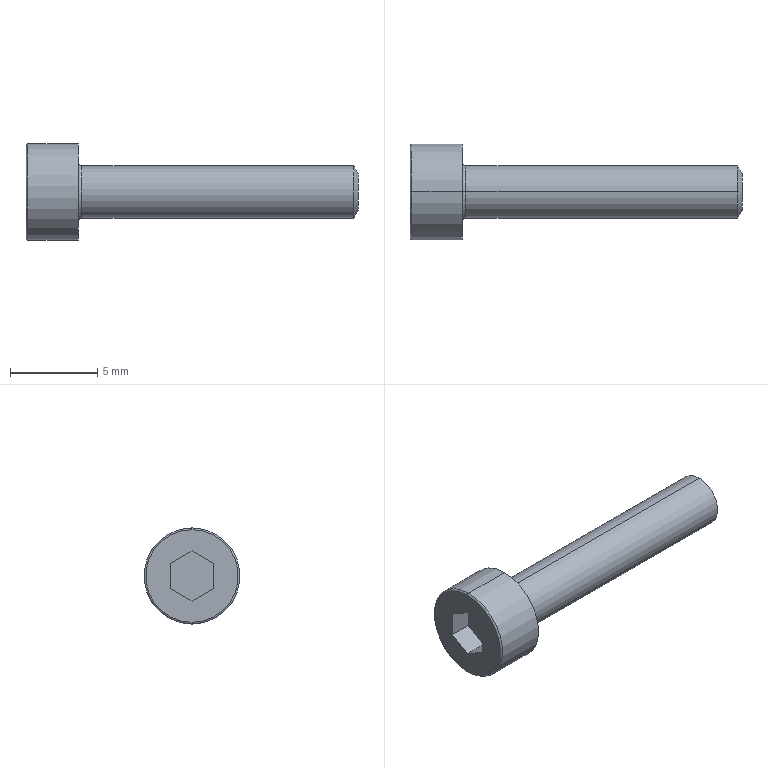Part | STEP file | 1 solid | 20 faces | box 19 x 5.5 x 5.5 mm | volume 177.003 mm3 | plane 10 | torus 4 | cylinder 4 | cone 2 | commonest cylinder face diameters 3 x2 5.5 x2
STEP:
#1=CARTESIAN_POINT('',(0.,0.,2.65));
#2=VERTEX_POINT('',#1);
#3=CARTESIAN_POINT('',(0.,0.,-2.65));
#4=VERTEX_POINT('',#3);
#5=CARTESIAN_POINT('',(0.,0.,0.));
#6=DIRECTION('',(-1.,0.,0.));
#7=DIRECTION('',(0.,0.,-1.));
#8=AXIS2_PLACEMENT_3D('',#5,#6,#7);
#9=CIRCLE('',#8,2.65);
#10=EDGE_CURVE('',#2,#4,#9,.T.);
#11=ORIENTED_EDGE('',*,*,#10,.F.);
#12=CARTESIAN_POINT('',(0.1,0.,2.75));
#13=VERTEX_POINT('',#12);
#14=CARTESIAN_POINT('',(0.1,0.,2.65));
#15=DIRECTION('',(0.,1.,0.));
#16=DIRECTION('',(0.,0.,1.));
#17=AXIS2_PLACEMENT_3D('',#14,#15,#16);
#18=CIRCLE('',#17,0.1);
#19=EDGE_CURVE('',#2,#13,#18,.T.);
#20=ORIENTED_EDGE('',*,*,#19,.T.);
#21=CARTESIAN_POINT('',(0.1,0.,-2.75));
#22=VERTEX_POINT('',#21);
#23=CARTESIAN_POINT('',(0.1,0.,0.));
#24=DIRECTION('',(1.,0.,0.));
#25=DIRECTION('',(0.,0.,-1.));
#26=AXIS2_PLACEMENT_3D('',#23,#24,#25);
#27=CIRCLE('',#26,2.75);
#28=EDGE_CURVE('',#22,#13,#27,.T.);
#29=ORIENTED_EDGE('',*,*,#28,.F.);
#30=CARTESIAN_POINT('',(0.1,0.,-2.65));
#31=DIRECTION('',(0.,-1.,0.));
#32=DIRECTION('',(0.,0.,-1.));
#33=AXIS2_PLACEMENT_3D('',#30,#31,#32);
#34=CIRCLE('',#33,0.1);
#35=EDGE_CURVE('',#4,#22,#34,.T.);
#36=ORIENTED_EDGE('',*,*,#35,.F.);
#37=EDGE_LOOP('',(#11,#20,#29,#36));
#38=FACE_OUTER_BOUND('',#37,.T.);
#39=CARTESIAN_POINT('',(0.1,0.,0.));
#40=DIRECTION('',(1.,0.,0.));
#41=DIRECTION('',(0.,0.,-1.));
#42=AXIS2_PLACEMENT_3D('',#39,#40,#41);
#43=TOROIDAL_SURFACE('',#42,2.65,0.1);
#44=ADVANCED_FACE('',(#38),#43,.T.);
#45=CARTESIAN_POINT('',(19.,0.,1.067));
#46=VERTEX_POINT('',#45);
#47=CARTESIAN_POINT('',(19.,0.,-1.067));
#48=VERTEX_POINT('',#47);
#49=CARTESIAN_POINT('',(19.,0.,0.));
#50=DIRECTION('',(-1.,0.,0.));
#51=DIRECTION('',(0.,0.,1.));
#52=AXIS2_PLACEMENT_3D('',#49,#50,#51);
#53=CIRCLE('',#52,1.067);
#54=EDGE_CURVE('',#46,#48,#53,.T.);
#55=ORIENTED_EDGE('',*,*,#54,.T.);
#56=CARTESIAN_POINT('',(18.75,0.,-1.5));
#57=VERTEX_POINT('',#56);
#58=CARTESIAN_POINT('',(18.75,0.,-1.5));
#59=DIRECTION('',(-0.5,0.,-0.866));
#60=VECTOR('',#59,1000.);
#61=LINE('',#58,#60);
#62=EDGE_CURVE('',#48,#57,#61,.T.);
#63=ORIENTED_EDGE('',*,*,#62,.T.);
#64=CARTESIAN_POINT('',(18.75,0.,1.5));
#65=VERTEX_POINT('',#64);
#66=CARTESIAN_POINT('',(18.75,0.,0.));
#67=DIRECTION('',(-1.,0.,0.));
#68=DIRECTION('',(0.,0.,1.));
#69=AXIS2_PLACEMENT_3D('',#66,#67,#68);
#70=CIRCLE('',#69,1.5);
#71=EDGE_CURVE('',#65,#57,#70,.T.);
#72=ORIENTED_EDGE('',*,*,#71,.F.);
#73=CARTESIAN_POINT('',(18.75,0.,1.5));
#74=DIRECTION('',(-0.5,0.,0.866));
#75=VECTOR('',#74,1000.);
#76=LINE('',#73,#75);
#77=EDGE_CURVE('',#46,#65,#76,.T.);
#78=ORIENTED_EDGE('',*,*,#77,.F.);
#79=EDGE_LOOP('',(#55,#63,#72,#78));
#80=FACE_OUTER_BOUND('',#79,.T.);
#81=CARTESIAN_POINT('',(18.75,0.,0.));
#82=DIRECTION('',(-1.,0.,0.));
#83=DIRECTION('',(0.,0.,1.));
#84=AXIS2_PLACEMENT_3D('',#81,#82,#83);
#85=CONICAL_SURFACE('',#84,1.5,1.047);
#86=ADVANCED_FACE('',(#80),#85,.T.);
#87=CARTESIAN_POINT('',(3.,0.,-1.7));
#88=VERTEX_POINT('',#87);
#89=CARTESIAN_POINT('',(3.,0.,1.7));
#90=VERTEX_POINT('',#89);
#91=CARTESIAN_POINT('',(3.,0.,0.));
#92=DIRECTION('',(-1.,0.,0.));
#93=DIRECTION('',(0.,0.,1.));
#94=AXIS2_PLACEMENT_3D('',#91,#92,#93);
#95=CIRCLE('',#94,1.7);
#96=EDGE_CURVE('',#88,#90,#95,.T.);
#97=ORIENTED_EDGE('',*,*,#96,.F.);
#98=CARTESIAN_POINT('',(3.2,0.,-1.5));
#99=VERTEX_POINT('',#98);
#100=CARTESIAN_POINT('',(3.2,0.,-1.7));
#101=DIRECTION('',(0.,1.,0.));
#102=DIRECTION('',(0.,0.,1.));
#103=AXIS2_PLACEMENT_3D('',#100,#101,#102);
#104=CIRCLE('',#103,0.2);
#105=EDGE_CURVE('',#88,#99,#104,.T.);
#106=ORIENTED_EDGE('',*,*,#105,.T.);
#107=CARTESIAN_POINT('',(3.2,0.,1.5));
#108=VERTEX_POINT('',#107);
#109=CARTESIAN_POINT('',(3.2,0.,0.));
#110=DIRECTION('',(-1.,0.,0.));
#111=DIRECTION('',(0.,0.,1.));
#112=AXIS2_PLACEMENT_3D('',#109,#110,#111);
#113=CIRCLE('',#112,1.5);
#114=EDGE_CURVE('',#99,#108,#113,.T.);
#115=ORIENTED_EDGE('',*,*,#114,.T.);
#116=CARTESIAN_POINT('',(3.2,0.,1.7));
#117=DIRECTION('',(0.,-1.,0.));
#118=DIRECTION('',(0.,0.,-1.));
#119=AXIS2_PLACEMENT_3D('',#116,#117,#118);
#120=CIRCLE('',#119,0.2);
#121=EDGE_CURVE('',#90,#108,#120,.T.);
#122=ORIENTED_EDGE('',*,*,#121,.F.);
#123=EDGE_LOOP('',(#97,#106,#115,#122));
#124=FACE_OUTER_BOUND('',#123,.T.);
#125=CARTESIAN_POINT('',(3.2,0.,0.));
#126=DIRECTION('',(-1.,0.,0.));
#127=DIRECTION('',(0.,0.,1.));
#128=AXIS2_PLACEMENT_3D('',#125,#126,#127);
#129=TOROIDAL_SURFACE('',#128,1.7,0.2);
#130=ADVANCED_FACE('',(#124),#129,.F.);
#131=CARTESIAN_POINT('',(3.,0.,2.75));
#132=VERTEX_POINT('',#131);
#133=CARTESIAN_POINT('',(3.,0.,-2.75));
#134=VERTEX_POINT('',#133);
#135=CARTESIAN_POINT('',(3.,0.,0.));
#136=DIRECTION('',(-1.,0.,0.));
#137=DIRECTION('',(0.,0.,1.));
#138=AXIS2_PLACEMENT_3D('',#135,#136,#137);
#139=CIRCLE('',#138,2.75);
#140=EDGE_CURVE('',#132,#134,#139,.T.);
#141=ORIENTED_EDGE('',*,*,#140,.T.);
#142=CARTESIAN_POINT('',(0.,0.,-2.75));
#143=DIRECTION('',(-1.,0.,0.));
#144=VECTOR('',#143,1000.);
#145=LINE('',#142,#144);
#146=EDGE_CURVE('',#134,#22,#145,.T.);
#147=ORIENTED_EDGE('',*,*,#146,.T.);
#148=ORIENTED_EDGE('',*,*,#28,.T.);
#149=CARTESIAN_POINT('',(0.,0.,2.75));
#150=DIRECTION('',(-1.,0.,0.));
#151=VECTOR('',#150,1000.);
#152=LINE('',#149,#151);
#153=EDGE_CURVE('',#132,#13,#152,.T.);
#154=ORIENTED_EDGE('',*,*,#153,.F.);
#155=EDGE_LOOP('',(#141,#147,#148,#154));
#156=FACE_OUTER_BOUND('',#155,.T.);
#157=CARTESIAN_POINT('',(0.,0.,0.));
#158=DIRECTION('',(-1.,0.,0.));
#159=DIRECTION('',(0.,0.,1.));
#160=AXIS2_PLACEMENT_3D('',#157,#158,#159);
#161=CYLINDRICAL_SURFACE('',#160,2.75);
#162=ADVANCED_FACE('',(#156),#161,.T.);
#163=ORIENTED_EDGE('',*,*,#71,.T.);
#164=CARTESIAN_POINT('',(0.,0.,-1.5));
#165=DIRECTION('',(-1.,0.,0.));
#166=VECTOR('',#165,1000.);
#167=LINE('',#164,#166);
#168=EDGE_CURVE('',#57,#99,#167,.T.);
#169=ORIENTED_EDGE('',*,*,#168,.T.);
#170=CARTESIAN_POINT('',(3.2,0.,0.));
#171=DIRECTION('',(-1.,0.,0.));
#172=DIRECTION('',(0.,0.,1.));
#173=AXIS2_PLACEMENT_3D('',#170,#171,#172);
#174=CIRCLE('',#173,1.5);
#175=EDGE_CURVE('',#108,#99,#174,.T.);
#176=ORIENTED_EDGE('',*,*,#175,.F.);
#177=CARTESIAN_POINT('',(0.,0.,1.5));
#178=DIRECTION('',(-1.,0.,0.));
#179=VECTOR('',#178,1000.);
#180=LINE('',#177,#179);
#181=EDGE_CURVE('',#65,#108,#180,.T.);
#182=ORIENTED_EDGE('',*,*,#181,.F.);
#183=EDGE_LOOP('',(#163,#169,#176,#182));
#184=FACE_OUTER_BOUND('',#183,.T.);
#185=CARTESIAN_POINT('',(0.,0.,0.));
#186=DIRECTION('',(-1.,0.,0.));
#187=DIRECTION('',(0.,0.,1.));
#188=AXIS2_PLACEMENT_3D('',#185,#186,#187);
#189=CYLINDRICAL_SURFACE('',#188,1.5);
#190=ADVANCED_FACE('',(#184),#189,.T.);
#191=ORIENTED_EDGE('',*,*,#168,.F.);
#192=CARTESIAN_POINT('',(18.75,0.,0.));
#193=DIRECTION('',(-1.,0.,0.));
#194=DIRECTION('',(0.,0.,1.));
#195=AXIS2_PLACEMENT_3D('',#192,#193,#194);
#196=CIRCLE('',#195,1.5);
#197=EDGE_CURVE('',#57,#65,#196,.T.);
#198=ORIENTED_EDGE('',*,*,#197,.T.);
#199=ORIENTED_EDGE('',*,*,#181,.T.);
#200=ORIENTED_EDGE('',*,*,#114,.F.);
#201=EDGE_LOOP('',(#191,#198,#199,#200));
#202=FACE_OUTER_BOUND('',#201,.T.);
#203=CARTESIAN_POINT('',(0.,0.,0.));
#204=DIRECTION('',(-1.,0.,0.));
#205=DIRECTION('',(0.,0.,1.));
#206=AXIS2_PLACEMENT_3D('',#203,#204,#205);
#207=CYLINDRICAL_SURFACE('',#206,1.5);
#208=ADVANCED_FACE('',(#202),#207,.T.);
#209=CARTESIAN_POINT('',(0.,0.,0.));
#210=DIRECTION('',(-1.,0.,0.));
#211=DIRECTION('',(0.,0.,-1.));
#212=AXIS2_PLACEMENT_3D('',#209,#210,#211);
#213=CIRCLE('',#212,2.65);
#214=EDGE_CURVE('',#4,#2,#213,.T.);
#215=ORIENTED_EDGE('',*,*,#214,.T.);
#216=ORIENTED_EDGE('',*,*,#10,.T.);
#217=EDGE_LOOP('',(#215,#216));
#218=FACE_OUTER_BOUND('',#217,.T.);
#219=CARTESIAN_POINT('',(0.,0.,1.435));
#220=VERTEX_POINT('',#219);
#221=CARTESIAN_POINT('',(0.,1.243,0.7175));
#222=VERTEX_POINT('',#221);
#223=CARTESIAN_POINT('',(0.,0.,1.435));
#224=DIRECTION('',(0.,0.866,-0.5));
#225=VECTOR('',#224,1000.);
#226=LINE('',#223,#225);
#227=EDGE_CURVE('',#220,#222,#226,.T.);
#228=ORIENTED_EDGE('',*,*,#227,.F.);
#229=CARTESIAN_POINT('',(0.,-1.243,0.7175));
#230=VERTEX_POINT('',#229);
#231=CARTESIAN_POINT('',(0.,-1.243,0.7175));
#232=DIRECTION('',(0.,0.866,0.5));
#233=VECTOR('',#232,1000.);
#234=LINE('',#231,#233);
#235=EDGE_CURVE('',#230,#220,#234,.T.);
#236=ORIENTED_EDGE('',*,*,#235,.F.);
#237=CARTESIAN_POINT('',(0.,-1.243,-0.7175));
#238=VERTEX_POINT('',#237);
#239=CARTESIAN_POINT('',(0.,-1.243,-0.7175));
#240=DIRECTION('',(0.,0.,1.));
#241=VECTOR('',#240,1000.);
#242=LINE('',#239,#241);
#243=EDGE_CURVE('',#238,#230,#242,.T.);
#244=ORIENTED_EDGE('',*,*,#243,.F.);
#245=CARTESIAN_POINT('',(0.,0.,-1.435));
#246=VERTEX_POINT('',#245);
#247=CARTESIAN_POINT('',(0.,0.,-1.435));
#248=DIRECTION('',(0.,-0.866,0.5));
#249=VECTOR('',#248,1000.);
#250=LINE('',#247,#249);
#251=EDGE_CURVE('',#246,#238,#250,.T.);
#252=ORIENTED_EDGE('',*,*,#251,.F.);
#253=CARTESIAN_POINT('',(0.,1.243,-0.7175));
#254=VERTEX_POINT('',#253);
#255=CARTESIAN_POINT('',(0.,1.243,-0.7175));
#256=DIRECTION('',(0.,-0.866,-0.5));
#257=VECTOR('',#256,1000.);
#258=LINE('',#255,#257);
#259=EDGE_CURVE('',#254,#246,#258,.T.);
#260=ORIENTED_EDGE('',*,*,#259,.F.);
#261=CARTESIAN_POINT('',(0.,1.243,0.7175));
#262=DIRECTION('',(0.,0.,-1.));
#263=VECTOR('',#262,1000.);
#264=LINE('',#261,#263);
#265=EDGE_CURVE('',#222,#254,#264,.T.);
#266=ORIENTED_EDGE('',*,*,#265,.F.);
#267=EDGE_LOOP('',(#228,#236,#244,#252,#260,#266));
#268=FACE_BOUND('',#267,.T.);
#269=CARTESIAN_POINT('',(0.,0.,0.));
#270=DIRECTION('',(1.,0.,0.));
#271=DIRECTION('',(0.,0.,-1.));
#272=AXIS2_PLACEMENT_3D('',#269,#270,#271);
#273=PLANE('',#272);
#274=ADVANCED_FACE('',(#218,#268),#273,.F.);
#275=ORIENTED_EDGE('',*,*,#146,.F.);
#276=CARTESIAN_POINT('',(3.,0.,0.));
#277=DIRECTION('',(-1.,0.,0.));
#278=DIRECTION('',(0.,0.,1.));
#279=AXIS2_PLACEMENT_3D('',#276,#277,#278);
#280=CIRCLE('',#279,2.75);
#281=EDGE_CURVE('',#134,#132,#280,.T.);
#282=ORIENTED_EDGE('',*,*,#281,.T.);
#283=ORIENTED_EDGE('',*,*,#153,.T.);
#284=CARTESIAN_POINT('',(0.1,0.,0.));
#285=DIRECTION('',(1.,0.,0.));
#286=DIRECTION('',(0.,0.,-1.));
#287=AXIS2_PLACEMENT_3D('',#284,#285,#286);
#288=CIRCLE('',#287,2.75);
#289=EDGE_CURVE('',#13,#22,#288,.T.);
#290=ORIENTED_EDGE('',*,*,#289,.T.);
#291=EDGE_LOOP('',(#275,#282,#283,#290));
#292=FACE_OUTER_BOUND('',#291,.T.);
#293=CARTESIAN_POINT('',(0.,0.,0.));
#294=DIRECTION('',(-1.,0.,0.));
#295=DIRECTION('',(0.,0.,1.));
#296=AXIS2_PLACEMENT_3D('',#293,#294,#295);
#297=CYLINDRICAL_SURFACE('',#296,2.75);
#298=ADVANCED_FACE('',(#292),#297,.T.);
#299=ORIENTED_EDGE('',*,*,#140,.F.);
#300=ORIENTED_EDGE('',*,*,#281,.F.);
#301=EDGE_LOOP('',(#299,#300));
#302=FACE_OUTER_BOUND('',#301,.T.);
#303=CARTESIAN_POINT('',(3.,0.,0.));
#304=DIRECTION('',(-1.,0.,0.));
#305=DIRECTION('',(0.,0.,1.));
#306=AXIS2_PLACEMENT_3D('',#303,#304,#305);
#307=CIRCLE('',#306,1.7);
#308=EDGE_CURVE('',#90,#88,#307,.T.);
#309=ORIENTED_EDGE('',*,*,#308,.T.);
#310=ORIENTED_EDGE('',*,*,#96,.T.);
#311=EDGE_LOOP('',(#309,#310));
#312=FACE_BOUND('',#311,.T.);
#313=CARTESIAN_POINT('',(3.,2.75,0.));
#314=DIRECTION('',(-1.,0.,0.));
#315=DIRECTION('',(0.,0.,1.));
#316=AXIS2_PLACEMENT_3D('',#313,#314,#315);
#317=PLANE('',#316);
#318=ADVANCED_FACE('',(#302,#312),#317,.F.);
#319=ORIENTED_EDGE('',*,*,#105,.F.);
#320=ORIENTED_EDGE('',*,*,#308,.F.);
#321=ORIENTED_EDGE('',*,*,#121,.T.);
#322=ORIENTED_EDGE('',*,*,#175,.T.);
#323=EDGE_LOOP('',(#319,#320,#321,#322));
#324=FACE_OUTER_BOUND('',#323,.T.);
#325=CARTESIAN_POINT('',(3.2,0.,0.));
#326=DIRECTION('',(-1.,0.,0.));
#327=DIRECTION('',(0.,0.,1.));
#328=AXIS2_PLACEMENT_3D('',#325,#326,#327);
#329=TOROIDAL_SURFACE('',#328,1.7,0.2);
#330=ADVANCED_FACE('',(#324),#329,.F.);
#331=ORIENTED_EDGE('',*,*,#235,.T.);
#332=CARTESIAN_POINT('',(1.3,0.,1.435));
#333=VERTEX_POINT('',#332);
#334=CARTESIAN_POINT('',(1.3,0.,1.435));
#335=DIRECTION('',(-1.,0.,0.));
#336=VECTOR('',#335,1000.);
#337=LINE('',#334,#336);
#338=EDGE_CURVE('',#333,#220,#337,.T.);
#339=ORIENTED_EDGE('',*,*,#338,.F.);
#340=CARTESIAN_POINT('',(1.3,-1.243,0.7175));
#341=VERTEX_POINT('',#340);
#342=CARTESIAN_POINT('',(1.3,-1.243,0.7175));
#343=DIRECTION('',(0.,0.866,0.5));
#344=VECTOR('',#343,1000.);
#345=LINE('',#342,#344);
#346=EDGE_CURVE('',#341,#333,#345,.T.);
#347=ORIENTED_EDGE('',*,*,#346,.F.);
#348=CARTESIAN_POINT('',(1.3,-1.243,0.7175));
#349=DIRECTION('',(-1.,0.,0.));
#350=VECTOR('',#349,1000.);
#351=LINE('',#348,#350);
#352=EDGE_CURVE('',#341,#230,#351,.T.);
#353=ORIENTED_EDGE('',*,*,#352,.T.);
#354=EDGE_LOOP('',(#331,#339,#347,#353));
#355=FACE_OUTER_BOUND('',#354,.T.);
#356=CARTESIAN_POINT('',(1.3,-1.243,0.7175));
#357=DIRECTION('',(0.,-0.5,0.866));
#358=DIRECTION('',(0.,-0.866,-0.5));
#359=AXIS2_PLACEMENT_3D('',#356,#357,#358);
#360=PLANE('',#359);
#361=ADVANCED_FACE('',(#355),#360,.F.);
#362=ORIENTED_EDGE('',*,*,#243,.T.);
#363=ORIENTED_EDGE('',*,*,#352,.F.);
#364=CARTESIAN_POINT('',(1.3,-1.243,-0.7175));
#365=VERTEX_POINT('',#364);
#366=CARTESIAN_POINT('',(1.3,-1.243,-0.7175));
#367=DIRECTION('',(0.,0.,1.));
#368=VECTOR('',#367,1000.);
#369=LINE('',#366,#368);
#370=EDGE_CURVE('',#365,#341,#369,.T.);
#371=ORIENTED_EDGE('',*,*,#370,.F.);
#372=CARTESIAN_POINT('',(1.3,-1.243,-0.7175));
#373=DIRECTION('',(-1.,0.,0.));
#374=VECTOR('',#373,1000.);
#375=LINE('',#372,#374);
#376=EDGE_CURVE('',#365,#238,#375,.T.);
#377=ORIENTED_EDGE('',*,*,#376,.T.);
#378=EDGE_LOOP('',(#362,#363,#371,#377));
#379=FACE_OUTER_BOUND('',#378,.T.);
#380=CARTESIAN_POINT('',(1.3,-1.243,-0.7175));
#381=DIRECTION('',(0.,-1.,0.));
#382=DIRECTION('',(0.,0.,-1.));
#383=AXIS2_PLACEMENT_3D('',#380,#381,#382);
#384=PLANE('',#383);
#385=ADVANCED_FACE('',(#379),#384,.F.);
#386=ORIENTED_EDGE('',*,*,#251,.T.);
#387=ORIENTED_EDGE('',*,*,#376,.F.);
#388=CARTESIAN_POINT('',(1.3,0.,-1.435));
#389=VERTEX_POINT('',#388);
#390=CARTESIAN_POINT('',(1.3,0.,-1.435));
#391=DIRECTION('',(0.,-0.866,0.5));
#392=VECTOR('',#391,1000.);
#393=LINE('',#390,#392);
#394=EDGE_CURVE('',#389,#365,#393,.T.);
#395=ORIENTED_EDGE('',*,*,#394,.F.);
#396=CARTESIAN_POINT('',(1.3,0.,-1.435));
#397=DIRECTION('',(-1.,0.,0.));
#398=VECTOR('',#397,1000.);
#399=LINE('',#396,#398);
#400=EDGE_CURVE('',#389,#246,#399,.T.);
#401=ORIENTED_EDGE('',*,*,#400,.T.);
#402=EDGE_LOOP('',(#386,#387,#395,#401));
#403=FACE_OUTER_BOUND('',#402,.T.);
#404=CARTESIAN_POINT('',(1.3,0.,-1.435));
#405=DIRECTION('',(0.,-0.5,-0.866));
#406=DIRECTION('',(0.,0.866,-0.5));
#407=AXIS2_PLACEMENT_3D('',#404,#405,#406);
#408=PLANE('',#407);
#409=ADVANCED_FACE('',(#403),#408,.F.);
#410=ORIENTED_EDGE('',*,*,#259,.T.);
#411=ORIENTED_EDGE('',*,*,#400,.F.);
#412=CARTESIAN_POINT('',(1.3,1.243,-0.7175));
#413=VERTEX_POINT('',#412);
#414=CARTESIAN_POINT('',(1.3,1.243,-0.7175));
#415=DIRECTION('',(0.,-0.866,-0.5));
#416=VECTOR('',#415,1000.);
#417=LINE('',#414,#416);
#418=EDGE_CURVE('',#413,#389,#417,.T.);
#419=ORIENTED_EDGE('',*,*,#418,.F.);
#420=CARTESIAN_POINT('',(1.3,1.243,-0.7175));
#421=DIRECTION('',(-1.,0.,0.));
#422=VECTOR('',#421,1000.);
#423=LINE('',#420,#422);
#424=EDGE_CURVE('',#413,#254,#423,.T.);
#425=ORIENTED_EDGE('',*,*,#424,.T.);
#426=EDGE_LOOP('',(#410,#411,#419,#425));
#427=FACE_OUTER_BOUND('',#426,.T.);
#428=CARTESIAN_POINT('',(1.3,1.243,-0.7175));
#429=DIRECTION('',(0.,0.5,-0.866));
#430=DIRECTION('',(0.,0.866,0.5));
#431=AXIS2_PLACEMENT_3D('',#428,#429,#430);
#432=PLANE('',#431);
#433=ADVANCED_FACE('',(#427),#432,.F.);
#434=ORIENTED_EDGE('',*,*,#265,.T.);
#435=ORIENTED_EDGE('',*,*,#424,.F.);
#436=CARTESIAN_POINT('',(1.3,1.243,0.7175));
#437=VERTEX_POINT('',#436);
#438=CARTESIAN_POINT('',(1.3,1.243,0.7175));
#439=DIRECTION('',(0.,0.,-1.));
#440=VECTOR('',#439,1000.);
#441=LINE('',#438,#440);
#442=EDGE_CURVE('',#437,#413,#441,.T.);
#443=ORIENTED_EDGE('',*,*,#442,.F.);
#444=CARTESIAN_POINT('',(1.3,1.243,0.7175));
#445=DIRECTION('',(-1.,0.,0.));
#446=VECTOR('',#445,1000.);
#447=LINE('',#444,#446);
#448=EDGE_CURVE('',#437,#222,#447,.T.);
#449=ORIENTED_EDGE('',*,*,#448,.T.);
#450=EDGE_LOOP('',(#434,#435,#443,#449));
#451=FACE_OUTER_BOUND('',#450,.T.);
#452=CARTESIAN_POINT('',(1.3,1.243,0.7175));
#453=DIRECTION('',(0.,1.,0.));
#454=DIRECTION('',(0.,0.,1.));
#455=AXIS2_PLACEMENT_3D('',#452,#453,#454);
#456=PLANE('',#455);
#457=ADVANCED_FACE('',(#451),#456,.F.);
#458=ORIENTED_EDGE('',*,*,#227,.T.);
#459=ORIENTED_EDGE('',*,*,#448,.F.);
#460=CARTESIAN_POINT('',(1.3,0.,1.435));
#461=DIRECTION('',(0.,0.866,-0.5));
#462=VECTOR('',#461,1000.);
#463=LINE('',#460,#462);
#464=EDGE_CURVE('',#333,#437,#463,.T.);
#465=ORIENTED_EDGE('',*,*,#464,.F.);
#466=ORIENTED_EDGE('',*,*,#338,.T.);
#467=EDGE_LOOP('',(#458,#459,#465,#466));
#468=FACE_OUTER_BOUND('',#467,.T.);
#469=CARTESIAN_POINT('',(1.3,0.,1.435));
#470=DIRECTION('',(0.,0.5,0.866));
#471=DIRECTION('',(0.,-0.866,0.5));
#472=AXIS2_PLACEMENT_3D('',#469,#470,#471);
#473=PLANE('',#472);
#474=ADVANCED_FACE('',(#468),#473,.F.);
#475=ORIENTED_EDGE('',*,*,#346,.T.);
#476=ORIENTED_EDGE('',*,*,#464,.T.);
#477=ORIENTED_EDGE('',*,*,#442,.T.);
#478=ORIENTED_EDGE('',*,*,#418,.T.);
#479=ORIENTED_EDGE('',*,*,#394,.T.);
#480=ORIENTED_EDGE('',*,*,#370,.T.);
#481=EDGE_LOOP('',(#475,#476,#477,#478,#479,#480));
#482=FACE_OUTER_BOUND('',#481,.T.);
#483=CARTESIAN_POINT('',(1.3,-1.243,0.7175));
#484=DIRECTION('',(1.,0.,0.));
#485=DIRECTION('',(0.,0.,-1.));
#486=AXIS2_PLACEMENT_3D('',#483,#484,#485);
#487=PLANE('',#486);
#488=ADVANCED_FACE('',(#482),#487,.F.);
#489=ORIENTED_EDGE('',*,*,#62,.F.);
#490=CARTESIAN_POINT('',(19.,0.,0.));
#491=DIRECTION('',(-1.,0.,0.));
#492=DIRECTION('',(0.,0.,1.));
#493=AXIS2_PLACEMENT_3D('',#490,#491,#492);
#494=CIRCLE('',#493,1.067);
#495=EDGE_CURVE('',#48,#46,#494,.T.);
#496=ORIENTED_EDGE('',*,*,#495,.T.);
#497=ORIENTED_EDGE('',*,*,#77,.T.);
#498=ORIENTED_EDGE('',*,*,#197,.F.);
#499=EDGE_LOOP('',(#489,#496,#497,#498));
#500=FACE_OUTER_BOUND('',#499,.T.);
#501=CARTESIAN_POINT('',(18.75,0.,0.));
#502=DIRECTION('',(-1.,0.,0.));
#503=DIRECTION('',(0.,0.,1.));
#504=AXIS2_PLACEMENT_3D('',#501,#502,#503);
#505=CONICAL_SURFACE('',#504,1.5,1.047);
#506=ADVANCED_FACE('',(#500),#505,.T.);
#507=ORIENTED_EDGE('',*,*,#54,.F.);
#508=ORIENTED_EDGE('',*,*,#495,.F.);
#509=EDGE_LOOP('',(#507,#508));
#510=FACE_OUTER_BOUND('',#509,.T.);
#511=CARTESIAN_POINT('',(19.,1.5,0.));
#512=DIRECTION('',(-1.,0.,0.));
#513=DIRECTION('',(0.,0.,1.));
#514=AXIS2_PLACEMENT_3D('',#511,#512,#513);
#515=PLANE('',#514);
#516=ADVANCED_FACE('',(#510),#515,.F.);
#517=ORIENTED_EDGE('',*,*,#19,.F.);
#518=ORIENTED_EDGE('',*,*,#214,.F.);
#519=ORIENTED_EDGE('',*,*,#35,.T.);
#520=ORIENTED_EDGE('',*,*,#289,.F.);
#521=EDGE_LOOP('',(#517,#518,#519,#520));
#522=FACE_OUTER_BOUND('',#521,.T.);
#523=CARTESIAN_POINT('',(0.1,0.,0.));
#524=DIRECTION('',(1.,0.,0.));
#525=DIRECTION('',(0.,0.,-1.));
#526=AXIS2_PLACEMENT_3D('',#523,#524,#525);
#527=TOROIDAL_SURFACE('',#526,2.65,0.1);
#528=ADVANCED_FACE('',(#522),#527,.T.);
#529=CLOSED_SHELL('',(#44,#86,#130,#162,#190,#208,#274,#298,#318,#330,#361,#385,#409,#433,#457,#474,#488,#506,#516,#528));
#530=MANIFOLD_SOLID_BREP('',#529);
#531=CARTESIAN_POINT('',(0.,0.,0.));
#532=DIRECTION('',(0.,0.,1.));
#533=DIRECTION('',(1.,0.,0.));
#534=AXIS2_PLACEMENT_3D('',#531,#532,#533);
#535=(LENGTH_UNIT()NAMED_UNIT(*)SI_UNIT(.MILLI.,.METRE.));
#536=UNCERTAINTY_MEASURE_WITH_UNIT(LENGTH_MEASURE(0.00001),#535,'','');
#537=(NAMED_UNIT(*)PLANE_ANGLE_UNIT()SI_UNIT($,.RADIAN.));
#538=(NAMED_UNIT(*)SI_UNIT($,.STERADIAN.)SOLID_ANGLE_UNIT());
#539=(GEOMETRIC_REPRESENTATION_CONTEXT(3)GLOBAL_UNCERTAINTY_ASSIGNED_CONTEXT((#536))GLOBAL_UNIT_ASSIGNED_CONTEXT((#535,#537,#538))REPRESENTATION_CONTEXT('',''));
#540=ADVANCED_BREP_SHAPE_REPRESENTATION('',(#530,#534),#539);